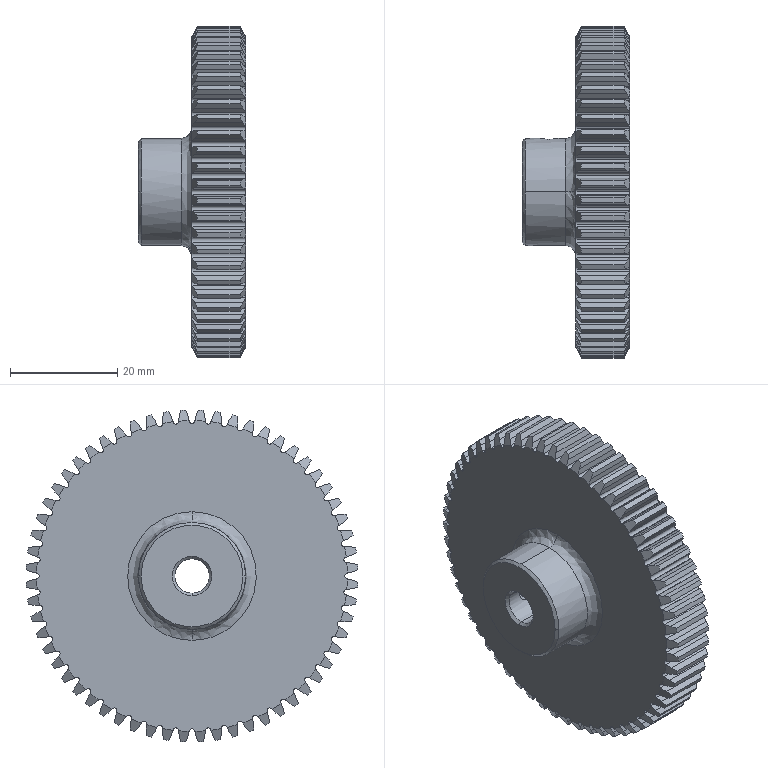Part | STEP file | 06-08 1-60 gear | 1 solid | 522 faces | box 20 x 61.958 x 61.958 mm | volume 30335 mm3 | plane 243 | cylinder 151 | cone 126 | spline 2 | commonest cylinder face diameters 1 x85 62 x60 3.3 x2 6.4 x2 20 x2